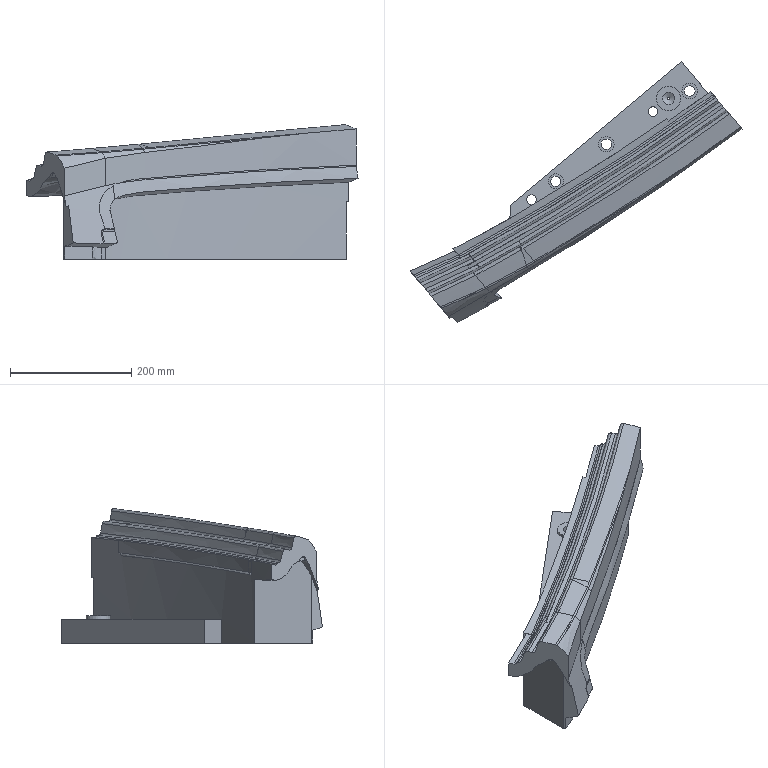Part | NX | features solid 2 | 1 solid | 114 faces | box 546.558 x 429.471 x 221.63 mm | volume 7622007 mm3 | spline 68 | plane 33 | cylinder 12 | cone 1 | commonest cylinder face diameters 16 x2 17.5 x2 25.5 x2 32 x2 17 x1 20 x1